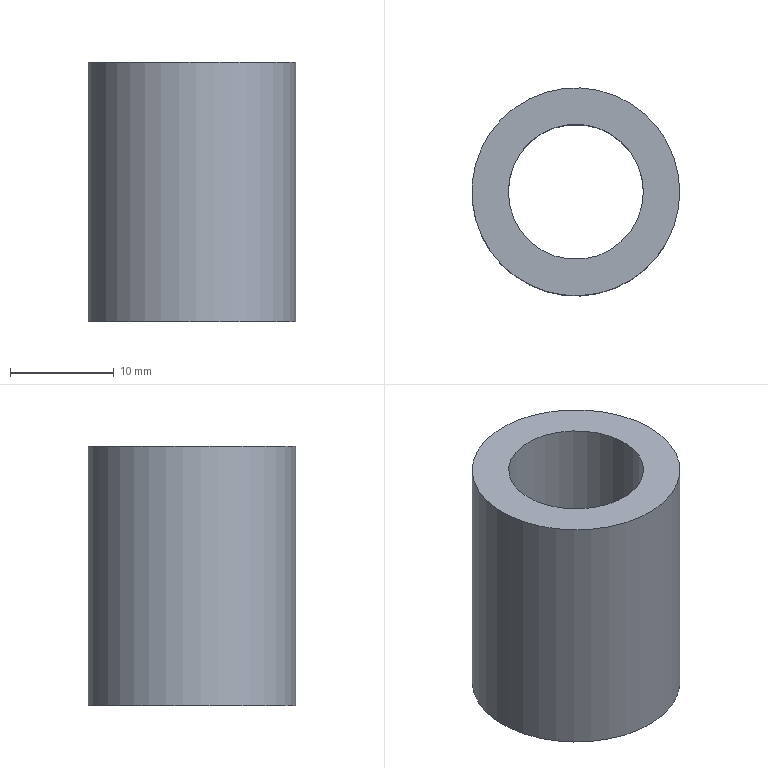Part | NX | features solid 2 | 1 solid | 4 faces | box 20 x 20 x 25 mm | volume 4536 mm3 | plane 2 | cylinder 2 | commonest cylinder face diameters 13 x1 20 x1
STEP:
#1=CARTESIAN_POINT('',(-479.,-240.,405.));
#2=VERTEX_POINT('',#1);
#3=CARTESIAN_POINT('',(-472.5,-240.,405.));
#4=DIRECTION('',(0.,0.,-1.));
#5=DIRECTION('',(-1.,0.,0.));
#6=AXIS2_PLACEMENT_3D('',#3,#4,#5);
#7=CIRCLE('',#6,6.5);
#8=EDGE_CURVE('',#2,#2,#7,.T.);
#9=ORIENTED_EDGE('',*,*,#8,.T.);
#10=EDGE_LOOP('',(#9));
#11=FACE_BOUND('',#10,.T.);
#12=CARTESIAN_POINT('',(-462.5,-240.,405.));
#13=VERTEX_POINT('',#12);
#14=CARTESIAN_POINT('',(-472.5,-240.,405.));
#15=DIRECTION('',(0.,0.,-1.));
#16=DIRECTION('',(1.,0.,0.));
#17=AXIS2_PLACEMENT_3D('',#14,#15,#16);
#18=CIRCLE('',#17,10.);
#19=EDGE_CURVE('',#13,#13,#18,.T.);
#20=ORIENTED_EDGE('',*,*,#19,.F.);
#21=EDGE_LOOP('',(#20));
#22=FACE_BOUND('',#21,.T.);
#23=CARTESIAN_POINT('',(-472.5,-240.,405.));
#24=DIRECTION('',(0.,0.,-1.));
#25=DIRECTION('',(1.,0.,0.));
#26=AXIS2_PLACEMENT_3D('',#23,#24,#25);
#27=PLANE('',#26);
#28=ADVANCED_FACE('',(#11,#22),#27,.F.);
#29=CARTESIAN_POINT('',(-479.,-240.,380.));
#30=VERTEX_POINT('',#29);
#31=CARTESIAN_POINT('',(-472.5,-240.,380.));
#32=DIRECTION('',(0.,0.,-1.));
#33=DIRECTION('',(-1.,0.,0.));
#34=AXIS2_PLACEMENT_3D('',#31,#32,#33);
#35=CIRCLE('',#34,6.5);
#36=EDGE_CURVE('',#30,#30,#35,.T.);
#37=ORIENTED_EDGE('',*,*,#36,.F.);
#38=EDGE_LOOP('',(#37));
#39=FACE_BOUND('',#38,.T.);
#40=CARTESIAN_POINT('',(-462.5,-240.,380.));
#41=VERTEX_POINT('',#40);
#42=CARTESIAN_POINT('',(-472.5,-240.,380.));
#43=DIRECTION('',(0.,0.,-1.));
#44=DIRECTION('',(1.,0.,0.));
#45=AXIS2_PLACEMENT_3D('',#42,#43,#44);
#46=CIRCLE('',#45,10.);
#47=EDGE_CURVE('',#41,#41,#46,.T.);
#48=ORIENTED_EDGE('',*,*,#47,.T.);
#49=EDGE_LOOP('',(#48));
#50=FACE_BOUND('',#49,.T.);
#51=CARTESIAN_POINT('',(-472.5,-240.,380.));
#52=DIRECTION('',(0.,0.,-1.));
#53=DIRECTION('',(1.,0.,0.));
#54=AXIS2_PLACEMENT_3D('',#51,#52,#53);
#55=PLANE('',#54);
#56=ADVANCED_FACE('',(#39,#50),#55,.T.);
#57=ORIENTED_EDGE('',*,*,#8,.F.);
#58=EDGE_LOOP('',(#57));
#59=FACE_BOUND('',#58,.T.);
#60=ORIENTED_EDGE('',*,*,#36,.T.);
#61=EDGE_LOOP('',(#60));
#62=FACE_BOUND('',#61,.T.);
#63=CARTESIAN_POINT('',(-472.5,-240.,380.));
#64=DIRECTION('',(0.,0.,1.));
#65=DIRECTION('',(-1.,0.,0.));
#66=AXIS2_PLACEMENT_3D('',#63,#64,#65);
#67=CYLINDRICAL_SURFACE('',#66,6.5);
#68=ADVANCED_FACE('',(#59,#62),#67,.F.);
#69=ORIENTED_EDGE('',*,*,#19,.T.);
#70=EDGE_LOOP('',(#69));
#71=FACE_BOUND('',#70,.T.);
#72=ORIENTED_EDGE('',*,*,#47,.F.);
#73=EDGE_LOOP('',(#72));
#74=FACE_BOUND('',#73,.T.);
#75=CARTESIAN_POINT('',(-472.5,-240.,380.));
#76=DIRECTION('',(0.,0.,1.));
#77=DIRECTION('',(-1.,0.,0.));
#78=AXIS2_PLACEMENT_3D('',#75,#76,#77);
#79=CYLINDRICAL_SURFACE('',#78,10.);
#80=ADVANCED_FACE('',(#71,#74),#79,.T.);
#81=CLOSED_SHELL('',(#28,#56,#68,#80));
#82=MANIFOLD_SOLID_BREP('',#81);
#83=(LENGTH_UNIT()NAMED_UNIT(*)SI_UNIT(.MILLI.,.METRE.));
#84=UNCERTAINTY_MEASURE_WITH_UNIT(LENGTH_MEASURE(0.00001),#83,'','');
#85=(NAMED_UNIT(*)PLANE_ANGLE_UNIT()SI_UNIT($,.RADIAN.));
#86=(NAMED_UNIT(*)SI_UNIT($,.STERADIAN.)SOLID_ANGLE_UNIT());
#87=(GEOMETRIC_REPRESENTATION_CONTEXT(3)GLOBAL_UNCERTAINTY_ASSIGNED_CONTEXT((#84))GLOBAL_UNIT_ASSIGNED_CONTEXT((#83,#85,#86))REPRESENTATION_CONTEXT('',''));
#88=ADVANCED_BREP_SHAPE_REPRESENTATION('',(#82),#87);